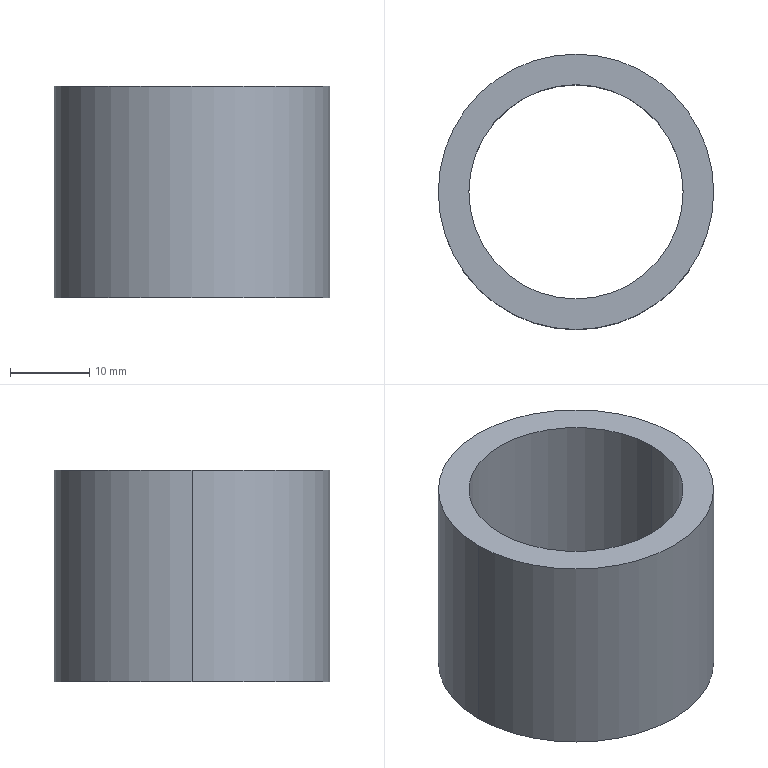Part | STEP file | 1 solid | 6 faces | box 34.7 x 34.7 x 26.7 mm | volume 9963 mm3 | cylinder 4 | plane 2 | commonest cylinder face diameters 27 x2 34.7 x2
STEP:
#1=CARTESIAN_POINT('',(0.,0.,0.));
#2=DIRECTION('',(0.,0.,1.));
#3=DIRECTION('',(1.,0.,0.));
#4=AXIS2_PLACEMENT_3D('',#1,#2,#3);
#5=CARTESIAN_POINT('',(-13.5,0.,0.));
#6=VERTEX_POINT('',#5);
#7=CARTESIAN_POINT('',(13.5,0.,0.));
#8=VERTEX_POINT('',#7);
#9=CARTESIAN_POINT('',(0.,0.,0.));
#10=DIRECTION('',(0.,0.,-1.));
#11=DIRECTION('',(-1.,0.,0.));
#12=AXIS2_PLACEMENT_3D('',#9,#10,#11);
#13=CIRCLE('',#12,13.5);
#14=CARTESIAN_POINT('',(13.5,0.,0.));
#15=DIRECTION('',(0.,0.,-1.));
#16=DIRECTION('',(-1.,0.,0.));
#17=AXIS2_PLACEMENT_3D('',#14,#15,#16);
#18=PLANE('',#17);
#19=CARTESIAN_POINT('',(13.5,0.));
#20=DIRECTION('',(1.,0.));
#21=AXIS2_PLACEMENT_2D('',#19,#20);
#22=CIRCLE('',#21,13.5);
#23=(GEOMETRIC_REPRESENTATION_CONTEXT(2)PARAMETRIC_REPRESENTATION_CONTEXT()REPRESENTATION_CONTEXT('',''));
#24=DEFINITIONAL_REPRESENTATION('',(#22),#23);
#25=PCURVE('',#18,#24);
#26=CARTESIAN_POINT('',(0.,0.,26.7));
#27=DIRECTION('',(0.,0.,-1.));
#28=DIRECTION('',(-1.,0.,0.));
#29=AXIS2_PLACEMENT_3D('',#26,#27,#28);
#30=CYLINDRICAL_SURFACE('',#29,13.5);
#31=CARTESIAN_POINT('',(0.,26.7));
#32=DIRECTION('',(1.,0.));
#33=VECTOR('',#32,1.);
#34=LINE('',#31,#33);
#35=(GEOMETRIC_REPRESENTATION_CONTEXT(2)PARAMETRIC_REPRESENTATION_CONTEXT()REPRESENTATION_CONTEXT('',''));
#36=DEFINITIONAL_REPRESENTATION('',(#34),#35);
#37=PCURVE('',#30,#36);
#38=SURFACE_CURVE('',#13,(#25,#37),.PCURVE_S1.);
#39=EDGE_CURVE('',#6,#8,#38,.T.);
#40=ORIENTED_EDGE('',*,*,#39,.F.);
#41=CARTESIAN_POINT('',(0.,0.,0.));
#42=DIRECTION('',(0.,0.,-1.));
#43=DIRECTION('',(-1.,0.,0.));
#44=AXIS2_PLACEMENT_3D('',#41,#42,#43);
#45=CIRCLE('',#44,13.5);
#46=CARTESIAN_POINT('',(13.5,0.));
#47=DIRECTION('',(1.,0.));
#48=AXIS2_PLACEMENT_2D('',#46,#47);
#49=CIRCLE('',#48,13.5);
#50=(GEOMETRIC_REPRESENTATION_CONTEXT(2)PARAMETRIC_REPRESENTATION_CONTEXT()REPRESENTATION_CONTEXT('',''));
#51=DEFINITIONAL_REPRESENTATION('',(#49),#50);
#52=PCURVE('',#18,#51);
#53=CARTESIAN_POINT('',(0.,0.,26.7));
#54=DIRECTION('',(0.,0.,-1.));
#55=DIRECTION('',(-1.,0.,0.));
#56=AXIS2_PLACEMENT_3D('',#53,#54,#55);
#57=CYLINDRICAL_SURFACE('',#56,13.5);
#58=CARTESIAN_POINT('',(0.,26.7));
#59=DIRECTION('',(1.,0.));
#60=VECTOR('',#59,1.);
#61=LINE('',#58,#60);
#62=(GEOMETRIC_REPRESENTATION_CONTEXT(2)PARAMETRIC_REPRESENTATION_CONTEXT()REPRESENTATION_CONTEXT('',''));
#63=DEFINITIONAL_REPRESENTATION('',(#61),#62);
#64=PCURVE('',#57,#63);
#65=SURFACE_CURVE('',#45,(#52,#64),.PCURVE_S1.);
#66=EDGE_CURVE('',#8,#6,#65,.T.);
#67=ORIENTED_EDGE('',*,*,#66,.F.);
#68=EDGE_LOOP('',(#40,#67));
#69=FACE_BOUND('',#68,.T.);
#70=CARTESIAN_POINT('',(-17.35,0.,0.));
#71=VERTEX_POINT('',#70);
#72=CARTESIAN_POINT('',(17.35,0.,0.));
#73=VERTEX_POINT('',#72);
#74=CARTESIAN_POINT('',(0.,0.,0.));
#75=DIRECTION('',(0.,0.,-1.));
#76=DIRECTION('',(-1.,0.,0.));
#77=AXIS2_PLACEMENT_3D('',#74,#75,#76);
#78=CIRCLE('',#77,17.35);
#79=CARTESIAN_POINT('',(13.5,0.));
#80=DIRECTION('',(1.,0.));
#81=AXIS2_PLACEMENT_2D('',#79,#80);
#82=CIRCLE('',#81,17.35);
#83=(GEOMETRIC_REPRESENTATION_CONTEXT(2)PARAMETRIC_REPRESENTATION_CONTEXT()REPRESENTATION_CONTEXT('',''));
#84=DEFINITIONAL_REPRESENTATION('',(#82),#83);
#85=PCURVE('',#18,#84);
#86=CARTESIAN_POINT('',(0.,0.,26.7));
#87=DIRECTION('',(0.,0.,-1.));
#88=DIRECTION('',(-1.,0.,0.));
#89=AXIS2_PLACEMENT_3D('',#86,#87,#88);
#90=CYLINDRICAL_SURFACE('',#89,17.35);
#91=CARTESIAN_POINT('',(0.,26.7));
#92=DIRECTION('',(1.,0.));
#93=VECTOR('',#92,1.);
#94=LINE('',#91,#93);
#95=(GEOMETRIC_REPRESENTATION_CONTEXT(2)PARAMETRIC_REPRESENTATION_CONTEXT()REPRESENTATION_CONTEXT('',''));
#96=DEFINITIONAL_REPRESENTATION('',(#94),#95);
#97=PCURVE('',#90,#96);
#98=SURFACE_CURVE('',#78,(#85,#97),.PCURVE_S1.);
#99=EDGE_CURVE('',#71,#73,#98,.T.);
#100=ORIENTED_EDGE('',*,*,#99,.T.);
#101=CARTESIAN_POINT('',(0.,0.,0.));
#102=DIRECTION('',(0.,0.,-1.));
#103=DIRECTION('',(-1.,0.,0.));
#104=AXIS2_PLACEMENT_3D('',#101,#102,#103);
#105=CIRCLE('',#104,17.35);
#106=CARTESIAN_POINT('',(13.5,0.));
#107=DIRECTION('',(1.,0.));
#108=AXIS2_PLACEMENT_2D('',#106,#107);
#109=CIRCLE('',#108,17.35);
#110=(GEOMETRIC_REPRESENTATION_CONTEXT(2)PARAMETRIC_REPRESENTATION_CONTEXT()REPRESENTATION_CONTEXT('',''));
#111=DEFINITIONAL_REPRESENTATION('',(#109),#110);
#112=PCURVE('',#18,#111);
#113=CARTESIAN_POINT('',(0.,0.,26.7));
#114=DIRECTION('',(0.,0.,-1.));
#115=DIRECTION('',(-1.,0.,0.));
#116=AXIS2_PLACEMENT_3D('',#113,#114,#115);
#117=CYLINDRICAL_SURFACE('',#116,17.35);
#118=CARTESIAN_POINT('',(0.,26.7));
#119=DIRECTION('',(1.,0.));
#120=VECTOR('',#119,1.);
#121=LINE('',#118,#120);
#122=(GEOMETRIC_REPRESENTATION_CONTEXT(2)PARAMETRIC_REPRESENTATION_CONTEXT()REPRESENTATION_CONTEXT('',''));
#123=DEFINITIONAL_REPRESENTATION('',(#121),#122);
#124=PCURVE('',#117,#123);
#125=SURFACE_CURVE('',#105,(#112,#124),.PCURVE_S1.);
#126=EDGE_CURVE('',#73,#71,#125,.T.);
#127=ORIENTED_EDGE('',*,*,#126,.T.);
#128=EDGE_LOOP('',(#100,#127));
#129=FACE_BOUND('',#128,.T.);
#130=ADVANCED_FACE('',(#69,#129),#18,.T.);
#131=ORIENTED_EDGE('',*,*,#39,.F.);
#132=CARTESIAN_POINT('',(-13.5,0.,26.7));
#133=VERTEX_POINT('',#132);
#134=CARTESIAN_POINT('',(-13.5,0.,26.7));
#135=DIRECTION('',(0.,0.,-1.));
#136=VECTOR('',#135,1.);
#137=LINE('',#134,#136);
#138=CARTESIAN_POINT('',(0.,0.));
#139=DIRECTION('',(0.,1.));
#140=VECTOR('',#139,1.);
#141=LINE('',#138,#140);
#142=(GEOMETRIC_REPRESENTATION_CONTEXT(2)PARAMETRIC_REPRESENTATION_CONTEXT()REPRESENTATION_CONTEXT('',''));
#143=DEFINITIONAL_REPRESENTATION('',(#141),#142);
#144=PCURVE('',#30,#143);
#145=CARTESIAN_POINT('',(6.283,0.));
#146=DIRECTION('',(0.,1.));
#147=VECTOR('',#146,1.);
#148=LINE('',#145,#147);
#149=(GEOMETRIC_REPRESENTATION_CONTEXT(2)PARAMETRIC_REPRESENTATION_CONTEXT()REPRESENTATION_CONTEXT('',''));
#150=DEFINITIONAL_REPRESENTATION('',(#148),#149);
#151=PCURVE('',#57,#150);
#152=SURFACE_CURVE('',#137,(#144,#151),.PCURVE_S1.);
#153=EDGE_CURVE('',#133,#6,#152,.T.);
#154=ORIENTED_EDGE('',*,*,#153,.F.);
#155=CARTESIAN_POINT('',(13.5,0.,26.7));
#156=VERTEX_POINT('',#155);
#157=CARTESIAN_POINT('',(0.,0.,26.7));
#158=DIRECTION('',(0.,0.,-1.));
#159=DIRECTION('',(-1.,0.,0.));
#160=AXIS2_PLACEMENT_3D('',#157,#158,#159);
#161=CIRCLE('',#160,13.5);
#162=CARTESIAN_POINT('',(0.,0.));
#163=DIRECTION('',(1.,0.));
#164=VECTOR('',#163,1.);
#165=LINE('',#162,#164);
#166=(GEOMETRIC_REPRESENTATION_CONTEXT(2)PARAMETRIC_REPRESENTATION_CONTEXT()REPRESENTATION_CONTEXT('',''));
#167=DEFINITIONAL_REPRESENTATION('',(#165),#166);
#168=PCURVE('',#30,#167);
#169=CARTESIAN_POINT('',(17.35,0.,26.7));
#170=DIRECTION('',(0.,0.,1.));
#171=DIRECTION('',(1.,0.,0.));
#172=AXIS2_PLACEMENT_3D('',#169,#170,#171);
#173=PLANE('',#172);
#174=CARTESIAN_POINT('',(-30.85,0.));
#175=CARTESIAN_POINT('',(-30.85,23.383));
#176=CARTESIAN_POINT('',(-10.6,11.691));
#177=CARTESIAN_POINT('',(9.65,0.));
#178=CARTESIAN_POINT('',(-10.6,-11.691));
#179=CARTESIAN_POINT('',(-30.85,-23.383));
#180=CARTESIAN_POINT('',(-30.85,0.));
#181=(BOUNDED_CURVE()B_SPLINE_CURVE(2,(#174,#175,#176,#177,#178,#179,#180),.UNSPECIFIED.,.T.,.F.)B_SPLINE_CURVE_WITH_KNOTS((1,2,2,2,2,1),(-2.094,0.,2.094,4.189,6.283,8.378),.UNSPECIFIED.)CURVE()GEOMETRIC_REPRESENTATION_ITEM()RATIONAL_B_SPLINE_CURVE((1.,0.5,1.,0.5,1.,0.5,1.))REPRESENTATION_ITEM(''));
#182=(GEOMETRIC_REPRESENTATION_CONTEXT(2)PARAMETRIC_REPRESENTATION_CONTEXT()REPRESENTATION_CONTEXT('',''));
#183=DEFINITIONAL_REPRESENTATION('',(#181),#182);
#184=PCURVE('',#173,#183);
#185=SURFACE_CURVE('',#161,(#168,#184),.PCURVE_S1.);
#186=EDGE_CURVE('',#133,#156,#185,.T.);
#187=ORIENTED_EDGE('',*,*,#186,.T.);
#188=CARTESIAN_POINT('',(13.5,0.,26.7));
#189=DIRECTION('',(0.,0.,-1.));
#190=VECTOR('',#189,1.);
#191=LINE('',#188,#190);
#192=CARTESIAN_POINT('',(3.142,0.));
#193=DIRECTION('',(0.,1.));
#194=VECTOR('',#193,1.);
#195=LINE('',#192,#194);
#196=(GEOMETRIC_REPRESENTATION_CONTEXT(2)PARAMETRIC_REPRESENTATION_CONTEXT()REPRESENTATION_CONTEXT('',''));
#197=DEFINITIONAL_REPRESENTATION('',(#195),#196);
#198=PCURVE('',#30,#197);
#199=CARTESIAN_POINT('',(3.142,0.));
#200=DIRECTION('',(0.,1.));
#201=VECTOR('',#200,1.);
#202=LINE('',#199,#201);
#203=(GEOMETRIC_REPRESENTATION_CONTEXT(2)PARAMETRIC_REPRESENTATION_CONTEXT()REPRESENTATION_CONTEXT('',''));
#204=DEFINITIONAL_REPRESENTATION('',(#202),#203);
#205=PCURVE('',#57,#204);
#206=SURFACE_CURVE('',#191,(#198,#205),.PCURVE_S1.);
#207=EDGE_CURVE('',#156,#8,#206,.T.);
#208=ORIENTED_EDGE('',*,*,#207,.T.);
#209=EDGE_LOOP('',(#131,#154,#187,#208));
#210=FACE_BOUND('',#209,.F.);
#211=ADVANCED_FACE('',(#210),#30,.F.);
#212=CARTESIAN_POINT('',(-17.35,0.,26.7));
#213=VERTEX_POINT('',#212);
#214=CARTESIAN_POINT('',(17.35,0.,26.7));
#215=VERTEX_POINT('',#214);
#216=CARTESIAN_POINT('',(0.,0.,26.7));
#217=DIRECTION('',(0.,0.,-1.));
#218=DIRECTION('',(-1.,0.,0.));
#219=AXIS2_PLACEMENT_3D('',#216,#217,#218);
#220=CIRCLE('',#219,17.35);
#221=CARTESIAN_POINT('',(-34.7,0.));
#222=CARTESIAN_POINT('',(-34.7,30.051));
#223=CARTESIAN_POINT('',(-8.675,15.026));
#224=CARTESIAN_POINT('',(17.35,0.));
#225=CARTESIAN_POINT('',(-8.675,-15.026));
#226=CARTESIAN_POINT('',(-34.7,-30.051));
#227=CARTESIAN_POINT('',(-34.7,0.));
#228=(BOUNDED_CURVE()B_SPLINE_CURVE(2,(#221,#222,#223,#224,#225,#226,#227),.UNSPECIFIED.,.T.,.F.)B_SPLINE_CURVE_WITH_KNOTS((1,2,2,2,2,1),(-2.094,0.,2.094,4.189,6.283,8.378),.UNSPECIFIED.)CURVE()GEOMETRIC_REPRESENTATION_ITEM()RATIONAL_B_SPLINE_CURVE((1.,0.5,1.,0.5,1.,0.5,1.))REPRESENTATION_ITEM(''));
#229=(GEOMETRIC_REPRESENTATION_CONTEXT(2)PARAMETRIC_REPRESENTATION_CONTEXT()REPRESENTATION_CONTEXT('',''));
#230=DEFINITIONAL_REPRESENTATION('',(#228),#229);
#231=PCURVE('',#173,#230);
#232=CARTESIAN_POINT('',(0.,0.));
#233=DIRECTION('',(1.,0.));
#234=VECTOR('',#233,1.);
#235=LINE('',#232,#234);
#236=(GEOMETRIC_REPRESENTATION_CONTEXT(2)PARAMETRIC_REPRESENTATION_CONTEXT()REPRESENTATION_CONTEXT('',''));
#237=DEFINITIONAL_REPRESENTATION('',(#235),#236);
#238=PCURVE('',#90,#237);
#239=SURFACE_CURVE('',#220,(#231,#238),.PCURVE_S1.);
#240=EDGE_CURVE('',#213,#215,#239,.T.);
#241=ORIENTED_EDGE('',*,*,#240,.F.);
#242=CARTESIAN_POINT('',(0.,0.,26.7));
#243=DIRECTION('',(0.,0.,-1.));
#244=DIRECTION('',(-1.,0.,0.));
#245=AXIS2_PLACEMENT_3D('',#242,#243,#244);
#246=CIRCLE('',#245,17.35);
#247=CARTESIAN_POINT('',(-34.7,0.));
#248=CARTESIAN_POINT('',(-34.7,30.051));
#249=CARTESIAN_POINT('',(-8.675,15.026));
#250=CARTESIAN_POINT('',(17.35,0.));
#251=CARTESIAN_POINT('',(-8.675,-15.026));
#252=CARTESIAN_POINT('',(-34.7,-30.051));
#253=CARTESIAN_POINT('',(-34.7,0.));
#254=(BOUNDED_CURVE()B_SPLINE_CURVE(2,(#247,#248,#249,#250,#251,#252,#253),.UNSPECIFIED.,.T.,.F.)B_SPLINE_CURVE_WITH_KNOTS((1,2,2,2,2,1),(-2.094,0.,2.094,4.189,6.283,8.378),.UNSPECIFIED.)CURVE()GEOMETRIC_REPRESENTATION_ITEM()RATIONAL_B_SPLINE_CURVE((1.,0.5,1.,0.5,1.,0.5,1.))REPRESENTATION_ITEM(''));
#255=(GEOMETRIC_REPRESENTATION_CONTEXT(2)PARAMETRIC_REPRESENTATION_CONTEXT()REPRESENTATION_CONTEXT('',''));
#256=DEFINITIONAL_REPRESENTATION('',(#254),#255);
#257=PCURVE('',#173,#256);
#258=CARTESIAN_POINT('',(0.,0.));
#259=DIRECTION('',(1.,0.));
#260=VECTOR('',#259,1.);
#261=LINE('',#258,#260);
#262=(GEOMETRIC_REPRESENTATION_CONTEXT(2)PARAMETRIC_REPRESENTATION_CONTEXT()REPRESENTATION_CONTEXT('',''));
#263=DEFINITIONAL_REPRESENTATION('',(#261),#262);
#264=PCURVE('',#117,#263);
#265=SURFACE_CURVE('',#246,(#257,#264),.PCURVE_S1.);
#266=EDGE_CURVE('',#215,#213,#265,.T.);
#267=ORIENTED_EDGE('',*,*,#266,.F.);
#268=EDGE_LOOP('',(#241,#267));
#269=FACE_BOUND('',#268,.T.);
#270=ORIENTED_EDGE('',*,*,#186,.T.);
#271=CARTESIAN_POINT('',(0.,0.,26.7));
#272=DIRECTION('',(0.,0.,-1.));
#273=DIRECTION('',(-1.,0.,0.));
#274=AXIS2_PLACEMENT_3D('',#271,#272,#273);
#275=CIRCLE('',#274,13.5);
#276=CARTESIAN_POINT('',(-30.85,0.));
#277=CARTESIAN_POINT('',(-30.85,23.383));
#278=CARTESIAN_POINT('',(-10.6,11.691));
#279=CARTESIAN_POINT('',(9.65,0.));
#280=CARTESIAN_POINT('',(-10.6,-11.691));
#281=CARTESIAN_POINT('',(-30.85,-23.383));
#282=CARTESIAN_POINT('',(-30.85,0.));
#283=(BOUNDED_CURVE()B_SPLINE_CURVE(2,(#276,#277,#278,#279,#280,#281,#282),.UNSPECIFIED.,.T.,.F.)B_SPLINE_CURVE_WITH_KNOTS((1,2,2,2,2,1),(-2.094,0.,2.094,4.189,6.283,8.378),.UNSPECIFIED.)CURVE()GEOMETRIC_REPRESENTATION_ITEM()RATIONAL_B_SPLINE_CURVE((1.,0.5,1.,0.5,1.,0.5,1.))REPRESENTATION_ITEM(''));
#284=(GEOMETRIC_REPRESENTATION_CONTEXT(2)PARAMETRIC_REPRESENTATION_CONTEXT()REPRESENTATION_CONTEXT('',''));
#285=DEFINITIONAL_REPRESENTATION('',(#283),#284);
#286=PCURVE('',#173,#285);
#287=CARTESIAN_POINT('',(0.,0.));
#288=DIRECTION('',(1.,0.));
#289=VECTOR('',#288,1.);
#290=LINE('',#287,#289);
#291=(GEOMETRIC_REPRESENTATION_CONTEXT(2)PARAMETRIC_REPRESENTATION_CONTEXT()REPRESENTATION_CONTEXT('',''));
#292=DEFINITIONAL_REPRESENTATION('',(#290),#291);
#293=PCURVE('',#57,#292);
#294=SURFACE_CURVE('',#275,(#286,#293),.PCURVE_S1.);
#295=EDGE_CURVE('',#156,#133,#294,.T.);
#296=ORIENTED_EDGE('',*,*,#295,.T.);
#297=EDGE_LOOP('',(#270,#296));
#298=FACE_BOUND('',#297,.T.);
#299=ADVANCED_FACE('',(#269,#298),#173,.T.);
#300=CARTESIAN_POINT('',(17.35,0.,26.7));
#301=DIRECTION('',(0.,0.,-1.));
#302=VECTOR('',#301,1.);
#303=LINE('',#300,#302);
#304=CARTESIAN_POINT('',(3.142,0.));
#305=DIRECTION('',(0.,1.));
#306=VECTOR('',#305,1.);
#307=LINE('',#304,#306);
#308=(GEOMETRIC_REPRESENTATION_CONTEXT(2)PARAMETRIC_REPRESENTATION_CONTEXT()REPRESENTATION_CONTEXT('',''));
#309=DEFINITIONAL_REPRESENTATION('',(#307),#308);
#310=PCURVE('',#117,#309);
#311=CARTESIAN_POINT('',(3.142,0.));
#312=DIRECTION('',(0.,1.));
#313=VECTOR('',#312,1.);
#314=LINE('',#311,#313);
#315=(GEOMETRIC_REPRESENTATION_CONTEXT(2)PARAMETRIC_REPRESENTATION_CONTEXT()REPRESENTATION_CONTEXT('',''));
#316=DEFINITIONAL_REPRESENTATION('',(#314),#315);
#317=PCURVE('',#90,#316);
#318=SURFACE_CURVE('',#303,(#310,#317),.PCURVE_S1.);
#319=EDGE_CURVE('',#215,#73,#318,.T.);
#320=ORIENTED_EDGE('',*,*,#319,.F.);
#321=ORIENTED_EDGE('',*,*,#266,.T.);
#322=CARTESIAN_POINT('',(-17.35,0.,26.7));
#323=DIRECTION('',(0.,0.,-1.));
#324=VECTOR('',#323,1.);
#325=LINE('',#322,#324);
#326=CARTESIAN_POINT('',(6.283,0.));
#327=DIRECTION('',(0.,1.));
#328=VECTOR('',#327,1.);
#329=LINE('',#326,#328);
#330=(GEOMETRIC_REPRESENTATION_CONTEXT(2)PARAMETRIC_REPRESENTATION_CONTEXT()REPRESENTATION_CONTEXT('',''));
#331=DEFINITIONAL_REPRESENTATION('',(#329),#330);
#332=PCURVE('',#117,#331);
#333=CARTESIAN_POINT('',(0.,0.));
#334=DIRECTION('',(0.,1.));
#335=VECTOR('',#334,1.);
#336=LINE('',#333,#335);
#337=(GEOMETRIC_REPRESENTATION_CONTEXT(2)PARAMETRIC_REPRESENTATION_CONTEXT()REPRESENTATION_CONTEXT('',''));
#338=DEFINITIONAL_REPRESENTATION('',(#336),#337);
#339=PCURVE('',#90,#338);
#340=SURFACE_CURVE('',#325,(#332,#339),.PCURVE_S1.);
#341=EDGE_CURVE('',#213,#71,#340,.T.);
#342=ORIENTED_EDGE('',*,*,#341,.T.);
#343=ORIENTED_EDGE('',*,*,#126,.F.);
#344=EDGE_LOOP('',(#320,#321,#342,#343));
#345=FACE_BOUND('',#344,.T.);
#346=ADVANCED_FACE('',(#345),#117,.T.);
#347=ORIENTED_EDGE('',*,*,#240,.T.);
#348=ORIENTED_EDGE('',*,*,#319,.T.);
#349=ORIENTED_EDGE('',*,*,#99,.F.);
#350=ORIENTED_EDGE('',*,*,#341,.F.);
#351=EDGE_LOOP('',(#347,#348,#349,#350));
#352=FACE_BOUND('',#351,.T.);
#353=ADVANCED_FACE('',(#352),#90,.T.);
#354=ORIENTED_EDGE('',*,*,#153,.T.);
#355=ORIENTED_EDGE('',*,*,#66,.F.);
#356=ORIENTED_EDGE('',*,*,#207,.F.);
#357=ORIENTED_EDGE('',*,*,#295,.T.);
#358=EDGE_LOOP('',(#354,#355,#356,#357));
#359=FACE_BOUND('',#358,.F.);
#360=ADVANCED_FACE('',(#359),#57,.F.);
#361=CLOSED_SHELL('',(#130,#211,#299,#346,#353,#360));
#362=MANIFOLD_SOLID_BREP('',#361);
#363=(LENGTH_UNIT()NAMED_UNIT(*)SI_UNIT(.MILLI.,.METRE.));
#364=UNCERTAINTY_MEASURE_WITH_UNIT(LENGTH_MEASURE(0.0000001),#363,'','');
#365=(NAMED_UNIT(*)PLANE_ANGLE_UNIT()SI_UNIT($,.RADIAN.));
#366=(NAMED_UNIT(*)SI_UNIT($,.STERADIAN.)SOLID_ANGLE_UNIT());
#367=(GEOMETRIC_REPRESENTATION_CONTEXT(3)GLOBAL_UNCERTAINTY_ASSIGNED_CONTEXT((#364))GLOBAL_UNIT_ASSIGNED_CONTEXT((#363,#365,#366))REPRESENTATION_CONTEXT('',''));
#368=ADVANCED_BREP_SHAPE_REPRESENTATION('',(#4,#362),#367);